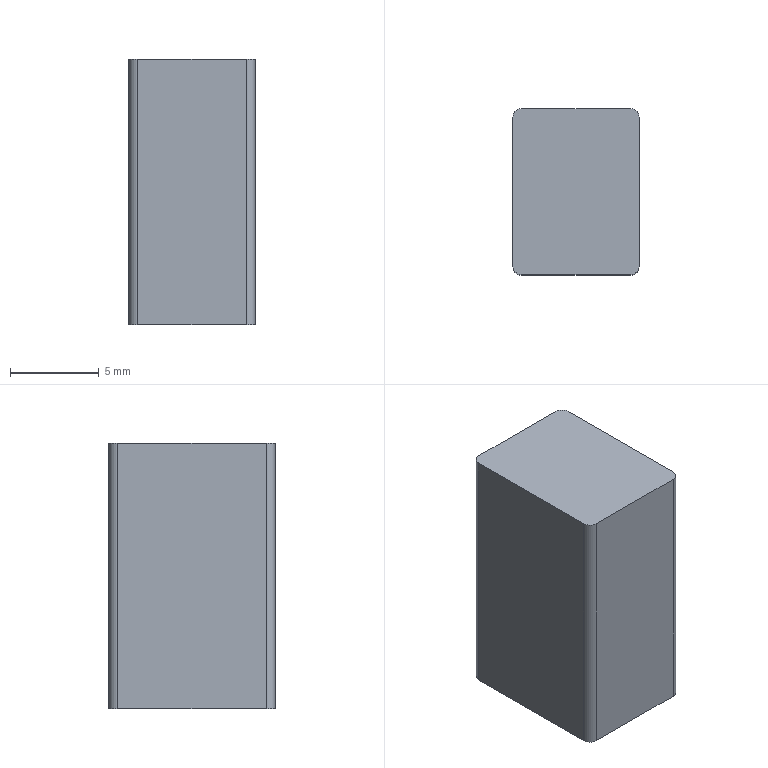Part | NX | features BREP 1 | 1 solid | 10 faces | box 7.124 x 9.391 x 15 mm | volume 1000 mm3 | plane 6 | cylinder 4 | commonest cylinder face diameters 1 x4
STEP:
#1=CARTESIAN_POINT('',(-3.062,4.695,-25.6));
#2=VERTEX_POINT('',#1);
#3=CARTESIAN_POINT('',(-3.562,4.195,-25.6));
#4=VERTEX_POINT('',#3);
#5=CARTESIAN_POINT('',(-3.062,4.195,-25.6));
#6=DIRECTION('',(0.,0.,1.));
#7=DIRECTION('',(1.,0.,0.));
#8=AXIS2_PLACEMENT_3D('',#5,#6,#7);
#9=CIRCLE('',#8,0.5);
#10=EDGE_CURVE('',#2,#4,#9,.T.);
#11=ORIENTED_EDGE('',*,*,#10,.F.);
#12=CARTESIAN_POINT('',(-3.062,4.695,-40.6));
#13=VERTEX_POINT('',#12);
#14=CARTESIAN_POINT('',(-3.062,4.695,-40.6));
#15=DIRECTION('',(0.,0.,1.));
#16=VECTOR('',#15,1000.);
#17=LINE('',#14,#16);
#18=EDGE_CURVE('',#13,#2,#17,.T.);
#19=ORIENTED_EDGE('',*,*,#18,.F.);
#20=CARTESIAN_POINT('',(-3.562,4.195,-40.6));
#21=VERTEX_POINT('',#20);
#22=CARTESIAN_POINT('',(-3.062,4.195,-40.6));
#23=DIRECTION('',(0.,0.,1.));
#24=DIRECTION('',(1.,0.,0.));
#25=AXIS2_PLACEMENT_3D('',#22,#23,#24);
#26=CIRCLE('',#25,0.5);
#27=EDGE_CURVE('',#13,#21,#26,.T.);
#28=ORIENTED_EDGE('',*,*,#27,.T.);
#29=CARTESIAN_POINT('',(-3.562,4.195,-40.6));
#30=DIRECTION('',(0.,0.,1.));
#31=VECTOR('',#30,1000.);
#32=LINE('',#29,#31);
#33=EDGE_CURVE('',#21,#4,#32,.T.);
#34=ORIENTED_EDGE('',*,*,#33,.T.);
#35=EDGE_LOOP('',(#11,#19,#28,#34));
#36=FACE_BOUND('',#35,.T.);
#37=CARTESIAN_POINT('',(-3.062,4.195,-40.6));
#38=DIRECTION('',(0.,0.,1.));
#39=DIRECTION('',(-1.,0.,0.));
#40=AXIS2_PLACEMENT_3D('',#37,#38,#39);
#41=CYLINDRICAL_SURFACE('',#40,0.5);
#42=ADVANCED_FACE('',(#36),#41,.T.);
#43=CARTESIAN_POINT('',(-3.562,-4.195,-25.6));
#44=VERTEX_POINT('',#43);
#45=CARTESIAN_POINT('',(-3.562,-4.195,-25.6));
#46=DIRECTION('',(0.,1.,0.));
#47=VECTOR('',#46,1000.);
#48=LINE('',#45,#47);
#49=EDGE_CURVE('',#44,#4,#48,.T.);
#50=ORIENTED_EDGE('',*,*,#49,.T.);
#51=ORIENTED_EDGE('',*,*,#33,.F.);
#52=CARTESIAN_POINT('',(-3.562,-4.195,-40.6));
#53=VERTEX_POINT('',#52);
#54=CARTESIAN_POINT('',(-3.562,-4.195,-40.6));
#55=DIRECTION('',(0.,1.,0.));
#56=VECTOR('',#55,1000.);
#57=LINE('',#54,#56);
#58=EDGE_CURVE('',#53,#21,#57,.T.);
#59=ORIENTED_EDGE('',*,*,#58,.F.);
#60=CARTESIAN_POINT('',(-3.562,-4.195,-40.6));
#61=DIRECTION('',(0.,0.,1.));
#62=VECTOR('',#61,1000.);
#63=LINE('',#60,#62);
#64=EDGE_CURVE('',#53,#44,#63,.T.);
#65=ORIENTED_EDGE('',*,*,#64,.T.);
#66=EDGE_LOOP('',(#50,#51,#59,#65));
#67=FACE_BOUND('',#66,.T.);
#68=CARTESIAN_POINT('',(-3.562,-4.195,-40.6));
#69=DIRECTION('',(1.,0.,0.));
#70=DIRECTION('',(0.,-1.,0.));
#71=AXIS2_PLACEMENT_3D('',#68,#69,#70);
#72=PLANE('',#71);
#73=ADVANCED_FACE('',(#67),#72,.F.);
#74=CARTESIAN_POINT('',(-3.062,-4.695,-25.6));
#75=VERTEX_POINT('',#74);
#76=CARTESIAN_POINT('',(-3.062,-4.195,-25.6));
#77=DIRECTION('',(0.,0.,1.));
#78=DIRECTION('',(1.,0.,0.));
#79=AXIS2_PLACEMENT_3D('',#76,#77,#78);
#80=CIRCLE('',#79,0.5);
#81=EDGE_CURVE('',#44,#75,#80,.T.);
#82=ORIENTED_EDGE('',*,*,#81,.F.);
#83=ORIENTED_EDGE('',*,*,#64,.F.);
#84=CARTESIAN_POINT('',(-3.062,-4.695,-40.6));
#85=VERTEX_POINT('',#84);
#86=CARTESIAN_POINT('',(-3.062,-4.195,-40.6));
#87=DIRECTION('',(0.,0.,1.));
#88=DIRECTION('',(1.,0.,0.));
#89=AXIS2_PLACEMENT_3D('',#86,#87,#88);
#90=CIRCLE('',#89,0.5);
#91=EDGE_CURVE('',#53,#85,#90,.T.);
#92=ORIENTED_EDGE('',*,*,#91,.T.);
#93=CARTESIAN_POINT('',(-3.062,-4.695,-40.6));
#94=DIRECTION('',(0.,0.,1.));
#95=VECTOR('',#94,1000.);
#96=LINE('',#93,#95);
#97=EDGE_CURVE('',#85,#75,#96,.T.);
#98=ORIENTED_EDGE('',*,*,#97,.T.);
#99=EDGE_LOOP('',(#82,#83,#92,#98));
#100=FACE_BOUND('',#99,.T.);
#101=CARTESIAN_POINT('',(-3.062,-4.195,-40.6));
#102=DIRECTION('',(0.,0.,1.));
#103=DIRECTION('',(-1.,0.,0.));
#104=AXIS2_PLACEMENT_3D('',#101,#102,#103);
#105=CYLINDRICAL_SURFACE('',#104,0.5);
#106=ADVANCED_FACE('',(#100),#105,.T.);
#107=CARTESIAN_POINT('',(3.062,-4.695,-25.6));
#108=VERTEX_POINT('',#107);
#109=CARTESIAN_POINT('',(3.062,-4.695,-25.6));
#110=DIRECTION('',(-1.,0.,0.));
#111=VECTOR('',#110,1000.);
#112=LINE('',#109,#111);
#113=EDGE_CURVE('',#108,#75,#112,.T.);
#114=ORIENTED_EDGE('',*,*,#113,.T.);
#115=ORIENTED_EDGE('',*,*,#97,.F.);
#116=CARTESIAN_POINT('',(3.062,-4.695,-40.6));
#117=VERTEX_POINT('',#116);
#118=CARTESIAN_POINT('',(3.062,-4.695,-40.6));
#119=DIRECTION('',(-1.,0.,0.));
#120=VECTOR('',#119,1000.);
#121=LINE('',#118,#120);
#122=EDGE_CURVE('',#117,#85,#121,.T.);
#123=ORIENTED_EDGE('',*,*,#122,.F.);
#124=CARTESIAN_POINT('',(3.062,-4.695,-40.6));
#125=DIRECTION('',(0.,0.,1.));
#126=VECTOR('',#125,1000.);
#127=LINE('',#124,#126);
#128=EDGE_CURVE('',#117,#108,#127,.T.);
#129=ORIENTED_EDGE('',*,*,#128,.T.);
#130=EDGE_LOOP('',(#114,#115,#123,#129));
#131=FACE_BOUND('',#130,.T.);
#132=CARTESIAN_POINT('',(3.062,-4.695,-40.6));
#133=DIRECTION('',(0.,1.,0.));
#134=DIRECTION('',(0.,0.,-1.));
#135=AXIS2_PLACEMENT_3D('',#132,#133,#134);
#136=PLANE('',#135);
#137=ADVANCED_FACE('',(#131),#136,.F.);
#138=CARTESIAN_POINT('',(3.562,-4.195,-25.6));
#139=VERTEX_POINT('',#138);
#140=CARTESIAN_POINT('',(3.062,-4.195,-25.6));
#141=DIRECTION('',(0.,0.,1.));
#142=DIRECTION('',(1.,0.,0.));
#143=AXIS2_PLACEMENT_3D('',#140,#141,#142);
#144=CIRCLE('',#143,0.5);
#145=EDGE_CURVE('',#108,#139,#144,.T.);
#146=ORIENTED_EDGE('',*,*,#145,.F.);
#147=ORIENTED_EDGE('',*,*,#128,.F.);
#148=CARTESIAN_POINT('',(3.562,-4.195,-40.6));
#149=VERTEX_POINT('',#148);
#150=CARTESIAN_POINT('',(3.062,-4.195,-40.6));
#151=DIRECTION('',(0.,0.,1.));
#152=DIRECTION('',(1.,0.,0.));
#153=AXIS2_PLACEMENT_3D('',#150,#151,#152);
#154=CIRCLE('',#153,0.5);
#155=EDGE_CURVE('',#117,#149,#154,.T.);
#156=ORIENTED_EDGE('',*,*,#155,.T.);
#157=CARTESIAN_POINT('',(3.562,-4.195,-40.6));
#158=DIRECTION('',(0.,0.,1.));
#159=VECTOR('',#158,1000.);
#160=LINE('',#157,#159);
#161=EDGE_CURVE('',#149,#139,#160,.T.);
#162=ORIENTED_EDGE('',*,*,#161,.T.);
#163=EDGE_LOOP('',(#146,#147,#156,#162));
#164=FACE_BOUND('',#163,.T.);
#165=CARTESIAN_POINT('',(3.062,-4.195,-40.6));
#166=DIRECTION('',(0.,0.,1.));
#167=DIRECTION('',(-1.,0.,0.));
#168=AXIS2_PLACEMENT_3D('',#165,#166,#167);
#169=CYLINDRICAL_SURFACE('',#168,0.5);
#170=ADVANCED_FACE('',(#164),#169,.T.);
#171=CARTESIAN_POINT('',(3.562,4.195,-25.6));
#172=VERTEX_POINT('',#171);
#173=CARTESIAN_POINT('',(3.562,4.195,-25.6));
#174=DIRECTION('',(0.,-1.,0.));
#175=VECTOR('',#174,1000.);
#176=LINE('',#173,#175);
#177=EDGE_CURVE('',#172,#139,#176,.T.);
#178=ORIENTED_EDGE('',*,*,#177,.T.);
#179=ORIENTED_EDGE('',*,*,#161,.F.);
#180=CARTESIAN_POINT('',(3.562,4.195,-40.6));
#181=VERTEX_POINT('',#180);
#182=CARTESIAN_POINT('',(3.562,4.195,-40.6));
#183=DIRECTION('',(0.,-1.,0.));
#184=VECTOR('',#183,1000.);
#185=LINE('',#182,#184);
#186=EDGE_CURVE('',#181,#149,#185,.T.);
#187=ORIENTED_EDGE('',*,*,#186,.F.);
#188=CARTESIAN_POINT('',(3.562,4.195,-40.6));
#189=DIRECTION('',(0.,0.,1.));
#190=VECTOR('',#189,1000.);
#191=LINE('',#188,#190);
#192=EDGE_CURVE('',#181,#172,#191,.T.);
#193=ORIENTED_EDGE('',*,*,#192,.T.);
#194=EDGE_LOOP('',(#178,#179,#187,#193));
#195=FACE_BOUND('',#194,.T.);
#196=CARTESIAN_POINT('',(3.562,4.195,-40.6));
#197=DIRECTION('',(-1.,0.,0.));
#198=DIRECTION('',(0.,1.,0.));
#199=AXIS2_PLACEMENT_3D('',#196,#197,#198);
#200=PLANE('',#199);
#201=ADVANCED_FACE('',(#195),#200,.F.);
#202=CARTESIAN_POINT('',(3.062,4.695,-25.6));
#203=VERTEX_POINT('',#202);
#204=CARTESIAN_POINT('',(3.062,4.195,-25.6));
#205=DIRECTION('',(0.,0.,1.));
#206=DIRECTION('',(1.,0.,0.));
#207=AXIS2_PLACEMENT_3D('',#204,#205,#206);
#208=CIRCLE('',#207,0.5);
#209=EDGE_CURVE('',#172,#203,#208,.T.);
#210=ORIENTED_EDGE('',*,*,#209,.F.);
#211=ORIENTED_EDGE('',*,*,#192,.F.);
#212=CARTESIAN_POINT('',(3.062,4.695,-40.6));
#213=VERTEX_POINT('',#212);
#214=CARTESIAN_POINT('',(3.062,4.195,-40.6));
#215=DIRECTION('',(0.,0.,1.));
#216=DIRECTION('',(1.,0.,0.));
#217=AXIS2_PLACEMENT_3D('',#214,#215,#216);
#218=CIRCLE('',#217,0.5);
#219=EDGE_CURVE('',#181,#213,#218,.T.);
#220=ORIENTED_EDGE('',*,*,#219,.T.);
#221=CARTESIAN_POINT('',(3.062,4.695,-40.6));
#222=DIRECTION('',(0.,0.,1.));
#223=VECTOR('',#222,1000.);
#224=LINE('',#221,#223);
#225=EDGE_CURVE('',#213,#203,#224,.T.);
#226=ORIENTED_EDGE('',*,*,#225,.T.);
#227=EDGE_LOOP('',(#210,#211,#220,#226));
#228=FACE_BOUND('',#227,.T.);
#229=CARTESIAN_POINT('',(3.062,4.195,-40.6));
#230=DIRECTION('',(0.,0.,1.));
#231=DIRECTION('',(-1.,0.,0.));
#232=AXIS2_PLACEMENT_3D('',#229,#230,#231);
#233=CYLINDRICAL_SURFACE('',#232,0.5);
#234=ADVANCED_FACE('',(#228),#233,.T.);
#235=CARTESIAN_POINT('',(-3.062,4.695,-25.6));
#236=DIRECTION('',(1.,0.,0.));
#237=VECTOR('',#236,1000.);
#238=LINE('',#235,#237);
#239=EDGE_CURVE('',#2,#203,#238,.T.);
#240=ORIENTED_EDGE('',*,*,#239,.T.);
#241=ORIENTED_EDGE('',*,*,#225,.F.);
#242=CARTESIAN_POINT('',(-3.062,4.695,-40.6));
#243=DIRECTION('',(1.,0.,0.));
#244=VECTOR('',#243,1000.);
#245=LINE('',#242,#244);
#246=EDGE_CURVE('',#13,#213,#245,.T.);
#247=ORIENTED_EDGE('',*,*,#246,.F.);
#248=ORIENTED_EDGE('',*,*,#18,.T.);
#249=EDGE_LOOP('',(#240,#241,#247,#248));
#250=FACE_BOUND('',#249,.T.);
#251=CARTESIAN_POINT('',(-3.062,4.695,-40.6));
#252=DIRECTION('',(0.,-1.,0.));
#253=DIRECTION('',(0.,0.,1.));
#254=AXIS2_PLACEMENT_3D('',#251,#252,#253);
#255=PLANE('',#254);
#256=ADVANCED_FACE('',(#250),#255,.F.);
#257=ORIENTED_EDGE('',*,*,#27,.F.);
#258=ORIENTED_EDGE('',*,*,#246,.T.);
#259=ORIENTED_EDGE('',*,*,#219,.F.);
#260=ORIENTED_EDGE('',*,*,#186,.T.);
#261=ORIENTED_EDGE('',*,*,#155,.F.);
#262=ORIENTED_EDGE('',*,*,#122,.T.);
#263=ORIENTED_EDGE('',*,*,#91,.F.);
#264=ORIENTED_EDGE('',*,*,#58,.T.);
#265=EDGE_LOOP('',(#257,#258,#259,#260,#261,#262,#263,#264));
#266=FACE_BOUND('',#265,.T.);
#267=CARTESIAN_POINT('',(-3.062,4.195,-40.6));
#268=DIRECTION('',(0.,0.,1.));
#269=DIRECTION('',(-1.,0.,0.));
#270=AXIS2_PLACEMENT_3D('',#267,#268,#269);
#271=PLANE('',#270);
#272=ADVANCED_FACE('',(#266),#271,.F.);
#273=ORIENTED_EDGE('',*,*,#10,.T.);
#274=ORIENTED_EDGE('',*,*,#49,.F.);
#275=ORIENTED_EDGE('',*,*,#81,.T.);
#276=ORIENTED_EDGE('',*,*,#113,.F.);
#277=ORIENTED_EDGE('',*,*,#145,.T.);
#278=ORIENTED_EDGE('',*,*,#177,.F.);
#279=ORIENTED_EDGE('',*,*,#209,.T.);
#280=ORIENTED_EDGE('',*,*,#239,.F.);
#281=EDGE_LOOP('',(#273,#274,#275,#276,#277,#278,#279,#280));
#282=FACE_BOUND('',#281,.T.);
#283=CARTESIAN_POINT('',(-3.062,4.195,-25.6));
#284=DIRECTION('',(0.,0.,1.));
#285=DIRECTION('',(-1.,0.,0.));
#286=AXIS2_PLACEMENT_3D('',#283,#284,#285);
#287=PLANE('',#286);
#288=ADVANCED_FACE('',(#282),#287,.T.);
#289=CLOSED_SHELL('',(#42,#73,#106,#137,#170,#201,#234,#256,#272,#288));
#290=MANIFOLD_SOLID_BREP('',#289);
#291=(LENGTH_UNIT()NAMED_UNIT(*)SI_UNIT(.MILLI.,.METRE.));
#292=UNCERTAINTY_MEASURE_WITH_UNIT(LENGTH_MEASURE(0.00001),#291,'','');
#293=(NAMED_UNIT(*)PLANE_ANGLE_UNIT()SI_UNIT($,.RADIAN.));
#294=(NAMED_UNIT(*)SI_UNIT($,.STERADIAN.)SOLID_ANGLE_UNIT());
#295=(GEOMETRIC_REPRESENTATION_CONTEXT(3)GLOBAL_UNCERTAINTY_ASSIGNED_CONTEXT((#292))GLOBAL_UNIT_ASSIGNED_CONTEXT((#291,#293,#294))REPRESENTATION_CONTEXT('',''));
#296=ADVANCED_BREP_SHAPE_REPRESENTATION('',(#290),#295);